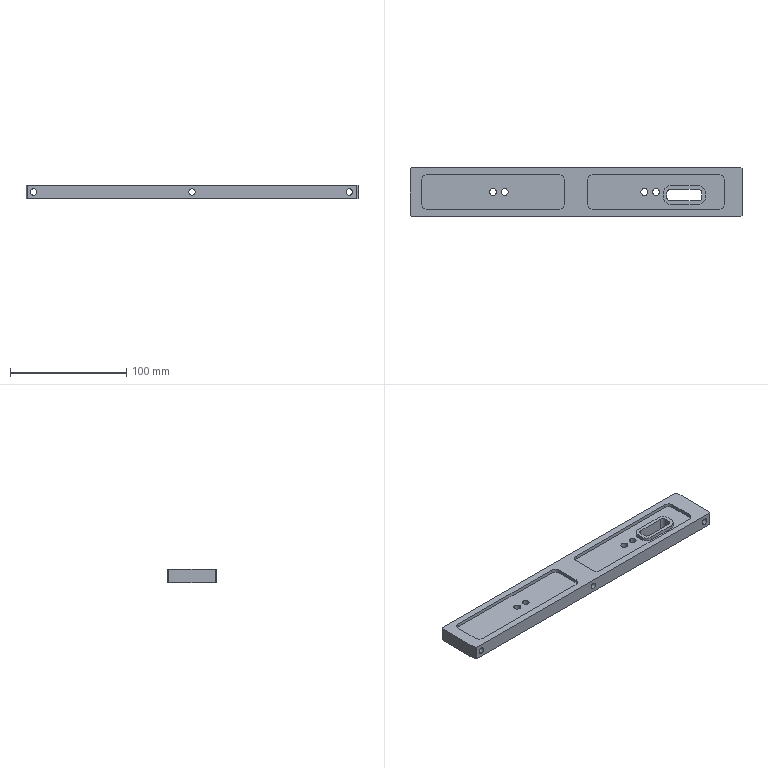Part | STEP file | J454-EBZ05-31-03-Part-1-1 | 1 solid | 68 faces | box 285 x 42 x 12 mm | volume 115201 mm3 | cylinder 36 | plane 32 | commonest cylinder face diameters 6 x12 10 x8 5.5 x6 9.5 x6 12 x4